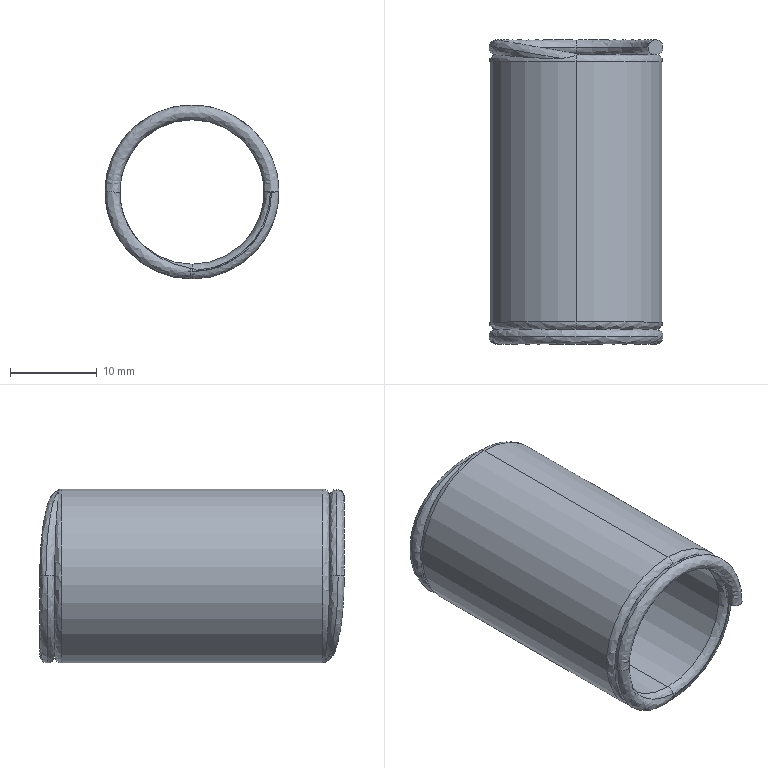Part | STEP file | TQ-DD-ul20_35_2_031010 | 1 solid | 31 faces | box 20 x 35 x 20 mm | volume 3226 mm3 | spline 23 | cylinder 4 | plane 4 | commonest cylinder face diameters 16.6 x2 20 x2